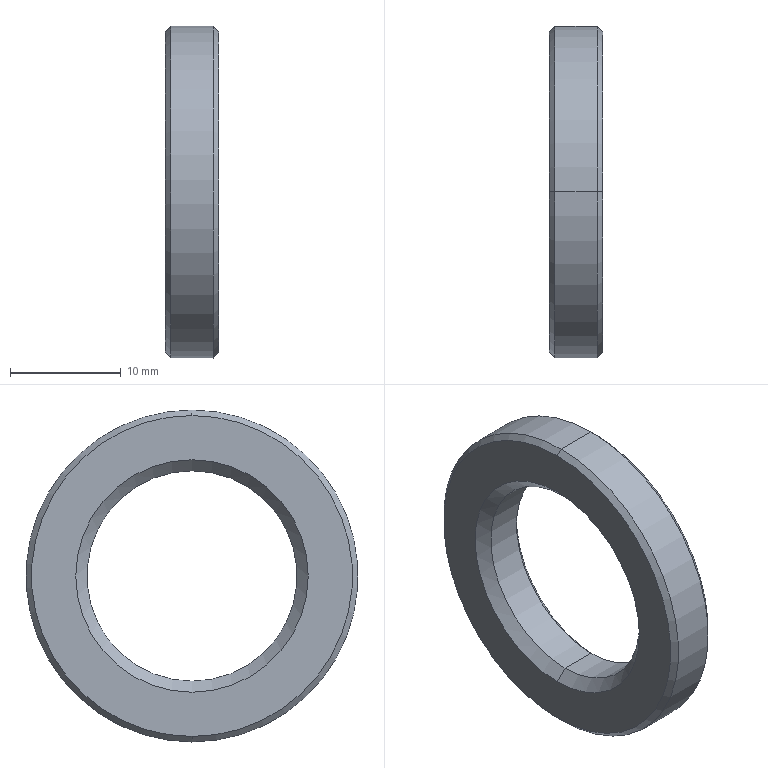Part | SolidWorks | features BaseBody 1 | 1 solid | 26 faces | box 4.8 x 30 x 30 mm | volume 1929 mm3 | cylinder 12 | cone 8 | plane 6 | commonest cylinder face diameters 2.1 x8 19 x2 30 x2
STEP:
#1=CARTESIAN_POINT('',(1.8,0.,15.));
#2=VERTEX_POINT('',#1);
#3=CARTESIAN_POINT('',(1.8,0.,-15.));
#4=VERTEX_POINT('',#3);
#5=CARTESIAN_POINT('',(1.8,0.,0.));
#6=DIRECTION('',(-1.,0.,0.));
#7=DIRECTION('',(0.,0.,1.));
#8=AXIS2_PLACEMENT_3D('',#5,#6,#7);
#9=CIRCLE('',#8,15.);
#10=EDGE_CURVE('',#2,#4,#9,.T.);
#11=ORIENTED_EDGE('',*,*,#10,.T.);
#12=CARTESIAN_POINT('',(-2.,0.,-15.));
#13=VERTEX_POINT('',#12);
#14=CARTESIAN_POINT('',(10.,0.,-15.));
#15=DIRECTION('',(-1.,0.,0.));
#16=VECTOR('',#15,1000.);
#17=LINE('',#14,#16);
#18=EDGE_CURVE('',#4,#13,#17,.T.);
#19=ORIENTED_EDGE('',*,*,#18,.T.);
#20=CARTESIAN_POINT('',(-2.,0.,15.));
#21=VERTEX_POINT('',#20);
#22=CARTESIAN_POINT('',(-2.,0.,0.));
#23=DIRECTION('',(1.,0.,0.));
#24=DIRECTION('',(0.,0.,1.));
#25=AXIS2_PLACEMENT_3D('',#22,#23,#24);
#26=CIRCLE('',#25,15.);
#27=EDGE_CURVE('',#13,#21,#26,.T.);
#28=ORIENTED_EDGE('',*,*,#27,.T.);
#29=CARTESIAN_POINT('',(10.,0.,15.));
#30=DIRECTION('',(-1.,0.,0.));
#31=VECTOR('',#30,1000.);
#32=LINE('',#29,#31);
#33=EDGE_CURVE('',#2,#21,#32,.T.);
#34=ORIENTED_EDGE('',*,*,#33,.F.);
#35=EDGE_LOOP('',(#11,#19,#28,#34));
#36=FACE_OUTER_BOUND('',#35,.T.);
#37=CARTESIAN_POINT('',(10.,0.,0.));
#38=DIRECTION('',(-1.,0.,0.));
#39=DIRECTION('',(0.,0.,1.));
#40=AXIS2_PLACEMENT_3D('',#37,#38,#39);
#41=CYLINDRICAL_SURFACE('',#40,15.);
#42=ADVANCED_FACE('',(#36),#41,.T.);
#43=CARTESIAN_POINT('',(2.3,0.,14.5));
#44=VERTEX_POINT('',#43);
#45=CARTESIAN_POINT('',(2.3,0.,-14.5));
#46=VERTEX_POINT('',#45);
#47=CARTESIAN_POINT('',(2.3,0.,0.));
#48=DIRECTION('',(-1.,0.,0.));
#49=DIRECTION('',(0.,0.,1.));
#50=AXIS2_PLACEMENT_3D('',#47,#48,#49);
#51=CIRCLE('',#50,14.5);
#52=EDGE_CURVE('',#44,#46,#51,.T.);
#53=ORIENTED_EDGE('',*,*,#52,.T.);
#54=CARTESIAN_POINT('',(1.8,0.,-15.));
#55=DIRECTION('',(-0.7071,0.,-0.7071));
#56=VECTOR('',#55,1000.);
#57=LINE('',#54,#56);
#58=EDGE_CURVE('',#46,#4,#57,.T.);
#59=ORIENTED_EDGE('',*,*,#58,.T.);
#60=ORIENTED_EDGE('',*,*,#10,.F.);
#61=CARTESIAN_POINT('',(1.8,0.,15.));
#62=DIRECTION('',(-0.7071,0.,0.7071));
#63=VECTOR('',#62,1000.);
#64=LINE('',#61,#63);
#65=EDGE_CURVE('',#44,#2,#64,.T.);
#66=ORIENTED_EDGE('',*,*,#65,.F.);
#67=EDGE_LOOP('',(#53,#59,#60,#66));
#68=FACE_OUTER_BOUND('',#67,.T.);
#69=CARTESIAN_POINT('',(1.8,0.,0.));
#70=DIRECTION('',(-1.,0.,0.));
#71=DIRECTION('',(0.,0.,1.));
#72=AXIS2_PLACEMENT_3D('',#69,#70,#71);
#73=CONICAL_SURFACE('',#72,15.,0.7854);
#74=ADVANCED_FACE('',(#68),#73,.T.);
#75=CARTESIAN_POINT('',(-2.5,0.,-14.5));
#76=VERTEX_POINT('',#75);
#77=CARTESIAN_POINT('',(-2.5,0.,14.5));
#78=VERTEX_POINT('',#77);
#79=CARTESIAN_POINT('',(-2.5,0.,0.));
#80=DIRECTION('',(1.,0.,0.));
#81=DIRECTION('',(0.,0.,-1.));
#82=AXIS2_PLACEMENT_3D('',#79,#80,#81);
#83=CIRCLE('',#82,14.5);
#84=EDGE_CURVE('',#76,#78,#83,.T.);
#85=ORIENTED_EDGE('',*,*,#84,.T.);
#86=CARTESIAN_POINT('',(-2.,0.,15.));
#87=DIRECTION('',(0.7071,0.,0.7071));
#88=VECTOR('',#87,1000.);
#89=LINE('',#86,#88);
#90=EDGE_CURVE('',#78,#21,#89,.T.);
#91=ORIENTED_EDGE('',*,*,#90,.T.);
#92=ORIENTED_EDGE('',*,*,#27,.F.);
#93=CARTESIAN_POINT('',(-2.,0.,-15.));
#94=DIRECTION('',(0.7071,0.,-0.7071));
#95=VECTOR('',#94,1000.);
#96=LINE('',#93,#95);
#97=EDGE_CURVE('',#76,#13,#96,.T.);
#98=ORIENTED_EDGE('',*,*,#97,.F.);
#99=EDGE_LOOP('',(#85,#91,#92,#98));
#100=FACE_OUTER_BOUND('',#99,.T.);
#101=CARTESIAN_POINT('',(-2.,0.,0.));
#102=DIRECTION('',(1.,0.,0.));
#103=DIRECTION('',(0.,0.,-1.));
#104=AXIS2_PLACEMENT_3D('',#101,#102,#103);
#105=CONICAL_SURFACE('',#104,15.,0.7854);
#106=ADVANCED_FACE('',(#100),#105,.T.);
#107=CARTESIAN_POINT('',(1.8,0.,9.5));
#108=VERTEX_POINT('',#107);
#109=CARTESIAN_POINT('',(1.8,0.,-9.5));
#110=VERTEX_POINT('',#109);
#111=CARTESIAN_POINT('',(1.8,0.,0.));
#112=DIRECTION('',(1.,0.,0.));
#113=DIRECTION('',(0.,0.,-1.));
#114=AXIS2_PLACEMENT_3D('',#111,#112,#113);
#115=CIRCLE('',#114,9.5);
#116=EDGE_CURVE('',#108,#110,#115,.T.);
#117=ORIENTED_EDGE('',*,*,#116,.F.);
#118=CARTESIAN_POINT('',(2.3,0.,10.));
#119=VERTEX_POINT('',#118);
#120=CARTESIAN_POINT('',(2.3,0.,10.));
#121=DIRECTION('',(0.7071,0.,0.7071));
#122=VECTOR('',#121,1000.);
#123=LINE('',#120,#122);
#124=EDGE_CURVE('',#108,#119,#123,.T.);
#125=ORIENTED_EDGE('',*,*,#124,.T.);
#126=CARTESIAN_POINT('',(2.3,0.,-10.));
#127=VERTEX_POINT('',#126);
#128=CARTESIAN_POINT('',(2.3,0.,0.));
#129=DIRECTION('',(-1.,0.,0.));
#130=DIRECTION('',(0.,0.,-1.));
#131=AXIS2_PLACEMENT_3D('',#128,#129,#130);
#132=CIRCLE('',#131,10.);
#133=EDGE_CURVE('',#127,#119,#132,.T.);
#134=ORIENTED_EDGE('',*,*,#133,.F.);
#135=CARTESIAN_POINT('',(2.3,0.,-10.));
#136=DIRECTION('',(0.7071,0.,-0.7071));
#137=VECTOR('',#136,1000.);
#138=LINE('',#135,#137);
#139=EDGE_CURVE('',#110,#127,#138,.T.);
#140=ORIENTED_EDGE('',*,*,#139,.F.);
#141=EDGE_LOOP('',(#117,#125,#134,#140));
#142=FACE_OUTER_BOUND('',#141,.T.);
#143=CARTESIAN_POINT('',(2.3,0.,0.));
#144=DIRECTION('',(1.,0.,0.));
#145=DIRECTION('',(0.,0.,-1.));
#146=AXIS2_PLACEMENT_3D('',#143,#144,#145);
#147=CONICAL_SURFACE('',#146,10.,0.7854);
#148=ADVANCED_FACE('',(#142),#147,.F.);
#149=CARTESIAN_POINT('',(2.3,-12.7,-1.05));
#150=VERTEX_POINT('',#149);
#151=CARTESIAN_POINT('',(2.3,-12.7,1.05));
#152=VERTEX_POINT('',#151);
#153=CARTESIAN_POINT('',(2.3,-12.7,0.));
#154=DIRECTION('',(-1.,0.,0.));
#155=DIRECTION('',(0.,0.,1.));
#156=AXIS2_PLACEMENT_3D('',#153,#154,#155);
#157=CIRCLE('',#156,1.05);
#158=EDGE_CURVE('',#150,#152,#157,.T.);
#159=ORIENTED_EDGE('',*,*,#158,.F.);
#160=CARTESIAN_POINT('',(-0.7,-12.7,-1.05));
#161=VERTEX_POINT('',#160);
#162=CARTESIAN_POINT('',(-0.7,-12.7,-1.05));
#163=DIRECTION('',(-1.,0.,0.));
#164=VECTOR('',#163,1000.);
#165=LINE('',#162,#164);
#166=EDGE_CURVE('',#150,#161,#165,.T.);
#167=ORIENTED_EDGE('',*,*,#166,.T.);
#168=CARTESIAN_POINT('',(-0.7,-12.7,1.05));
#169=VERTEX_POINT('',#168);
#170=CARTESIAN_POINT('',(-0.7,-12.7,0.));
#171=DIRECTION('',(1.,0.,0.));
#172=DIRECTION('',(0.,0.,1.));
#173=AXIS2_PLACEMENT_3D('',#170,#171,#172);
#174=CIRCLE('',#173,1.05);
#175=EDGE_CURVE('',#169,#161,#174,.T.);
#176=ORIENTED_EDGE('',*,*,#175,.F.);
#177=CARTESIAN_POINT('',(-0.7,-12.7,1.05));
#178=DIRECTION('',(-1.,0.,0.));
#179=VECTOR('',#178,1000.);
#180=LINE('',#177,#179);
#181=EDGE_CURVE('',#152,#169,#180,.T.);
#182=ORIENTED_EDGE('',*,*,#181,.F.);
#183=EDGE_LOOP('',(#159,#167,#176,#182));
#184=FACE_OUTER_BOUND('',#183,.T.);
#185=CARTESIAN_POINT('',(-0.7,-12.7,0.));
#186=DIRECTION('',(-1.,0.,0.));
#187=DIRECTION('',(0.,0.,1.));
#188=AXIS2_PLACEMENT_3D('',#185,#186,#187);
#189=CYLINDRICAL_SURFACE('',#188,1.05);
#190=ADVANCED_FACE('',(#184),#189,.F.);
#191=CARTESIAN_POINT('',(2.3,0.,-13.75));
#192=VERTEX_POINT('',#191);
#193=CARTESIAN_POINT('',(2.3,0.,-11.65));
#194=VERTEX_POINT('',#193);
#195=CARTESIAN_POINT('',(2.3,0.,-12.7));
#196=DIRECTION('',(-1.,0.,0.));
#197=DIRECTION('',(0.,0.,1.));
#198=AXIS2_PLACEMENT_3D('',#195,#196,#197);
#199=CIRCLE('',#198,1.05);
#200=EDGE_CURVE('',#192,#194,#199,.T.);
#201=ORIENTED_EDGE('',*,*,#200,.F.);
#202=CARTESIAN_POINT('',(-0.7,0.,-13.75));
#203=VERTEX_POINT('',#202);
#204=CARTESIAN_POINT('',(-0.7,0.,-13.75));
#205=DIRECTION('',(-1.,0.,0.));
#206=VECTOR('',#205,1000.);
#207=LINE('',#204,#206);
#208=EDGE_CURVE('',#192,#203,#207,.T.);
#209=ORIENTED_EDGE('',*,*,#208,.T.);
#210=CARTESIAN_POINT('',(-0.7,0.,-11.65));
#211=VERTEX_POINT('',#210);
#212=CARTESIAN_POINT('',(-0.7,0.,-12.7));
#213=DIRECTION('',(1.,0.,0.));
#214=DIRECTION('',(0.,0.,1.));
#215=AXIS2_PLACEMENT_3D('',#212,#213,#214);
#216=CIRCLE('',#215,1.05);
#217=EDGE_CURVE('',#211,#203,#216,.T.);
#218=ORIENTED_EDGE('',*,*,#217,.F.);
#219=CARTESIAN_POINT('',(-0.7,0.,-11.65));
#220=DIRECTION('',(-1.,0.,0.));
#221=VECTOR('',#220,1000.);
#222=LINE('',#219,#221);
#223=EDGE_CURVE('',#194,#211,#222,.T.);
#224=ORIENTED_EDGE('',*,*,#223,.F.);
#225=EDGE_LOOP('',(#201,#209,#218,#224));
#226=FACE_OUTER_BOUND('',#225,.T.);
#227=CARTESIAN_POINT('',(-0.7,0.,-12.7));
#228=DIRECTION('',(-1.,0.,0.));
#229=DIRECTION('',(0.,0.,1.));
#230=AXIS2_PLACEMENT_3D('',#227,#228,#229);
#231=CYLINDRICAL_SURFACE('',#230,1.05);
#232=ADVANCED_FACE('',(#226),#231,.F.);
#233=CARTESIAN_POINT('',(2.3,0.,11.65));
#234=VERTEX_POINT('',#233);
#235=CARTESIAN_POINT('',(2.3,0.,13.75));
#236=VERTEX_POINT('',#235);
#237=CARTESIAN_POINT('',(2.3,0.,12.7));
#238=DIRECTION('',(-1.,0.,0.));
#239=DIRECTION('',(0.,0.,1.));
#240=AXIS2_PLACEMENT_3D('',#237,#238,#239);
#241=CIRCLE('',#240,1.05);
#242=EDGE_CURVE('',#234,#236,#241,.T.);
#243=ORIENTED_EDGE('',*,*,#242,.F.);
#244=CARTESIAN_POINT('',(-0.7,0.,11.65));
#245=VERTEX_POINT('',#244);
#246=CARTESIAN_POINT('',(-0.7,0.,11.65));
#247=DIRECTION('',(-1.,0.,0.));
#248=VECTOR('',#247,1000.);
#249=LINE('',#246,#248);
#250=EDGE_CURVE('',#234,#245,#249,.T.);
#251=ORIENTED_EDGE('',*,*,#250,.T.);
#252=CARTESIAN_POINT('',(-0.7,0.,13.75));
#253=VERTEX_POINT('',#252);
#254=CARTESIAN_POINT('',(-0.7,0.,12.7));
#255=DIRECTION('',(1.,0.,0.));
#256=DIRECTION('',(0.,0.,1.));
#257=AXIS2_PLACEMENT_3D('',#254,#255,#256);
#258=CIRCLE('',#257,1.05);
#259=EDGE_CURVE('',#253,#245,#258,.T.);
#260=ORIENTED_EDGE('',*,*,#259,.F.);
#261=CARTESIAN_POINT('',(-0.7,0.,13.75));
#262=DIRECTION('',(-1.,0.,0.));
#263=VECTOR('',#262,1000.);
#264=LINE('',#261,#263);
#265=EDGE_CURVE('',#236,#253,#264,.T.);
#266=ORIENTED_EDGE('',*,*,#265,.F.);
#267=EDGE_LOOP('',(#243,#251,#260,#266));
#268=FACE_OUTER_BOUND('',#267,.T.);
#269=CARTESIAN_POINT('',(-0.7,0.,12.7));
#270=DIRECTION('',(-1.,0.,0.));
#271=DIRECTION('',(0.,0.,1.));
#272=AXIS2_PLACEMENT_3D('',#269,#270,#271);
#273=CYLINDRICAL_SURFACE('',#272,1.05);
#274=ADVANCED_FACE('',(#268),#273,.F.);
#275=CARTESIAN_POINT('',(2.3,12.7,-1.05));
#276=VERTEX_POINT('',#275);
#277=CARTESIAN_POINT('',(2.3,12.7,1.05));
#278=VERTEX_POINT('',#277);
#279=CARTESIAN_POINT('',(2.3,12.7,0.));
#280=DIRECTION('',(-1.,0.,0.));
#281=DIRECTION('',(0.,0.,1.));
#282=AXIS2_PLACEMENT_3D('',#279,#280,#281);
#283=CIRCLE('',#282,1.05);
#284=EDGE_CURVE('',#276,#278,#283,.T.);
#285=ORIENTED_EDGE('',*,*,#284,.F.);
#286=CARTESIAN_POINT('',(-0.7,12.7,-1.05));
#287=VERTEX_POINT('',#286);
#288=CARTESIAN_POINT('',(-0.7,12.7,-1.05));
#289=DIRECTION('',(-1.,0.,0.));
#290=VECTOR('',#289,1000.);
#291=LINE('',#288,#290);
#292=EDGE_CURVE('',#276,#287,#291,.T.);
#293=ORIENTED_EDGE('',*,*,#292,.T.);
#294=CARTESIAN_POINT('',(-0.7,12.7,1.05));
#295=VERTEX_POINT('',#294);
#296=CARTESIAN_POINT('',(-0.7,12.7,0.));
#297=DIRECTION('',(1.,0.,0.));
#298=DIRECTION('',(0.,0.,1.));
#299=AXIS2_PLACEMENT_3D('',#296,#297,#298);
#300=CIRCLE('',#299,1.05);
#301=EDGE_CURVE('',#295,#287,#300,.T.);
#302=ORIENTED_EDGE('',*,*,#301,.F.);
#303=CARTESIAN_POINT('',(-0.7,12.7,1.05));
#304=DIRECTION('',(-1.,0.,0.));
#305=VECTOR('',#304,1000.);
#306=LINE('',#303,#305);
#307=EDGE_CURVE('',#278,#295,#306,.T.);
#308=ORIENTED_EDGE('',*,*,#307,.F.);
#309=EDGE_LOOP('',(#285,#293,#302,#308));
#310=FACE_OUTER_BOUND('',#309,.T.);
#311=CARTESIAN_POINT('',(-0.7,12.7,0.));
#312=DIRECTION('',(-1.,0.,0.));
#313=DIRECTION('',(0.,0.,1.));
#314=AXIS2_PLACEMENT_3D('',#311,#312,#313);
#315=CYLINDRICAL_SURFACE('',#314,1.05);
#316=ADVANCED_FACE('',(#310),#315,.F.);
#317=CARTESIAN_POINT('',(-1.5,0.,-9.5));
#318=VERTEX_POINT('',#317);
#319=CARTESIAN_POINT('',(-1.5,0.,9.5));
#320=VERTEX_POINT('',#319);
#321=CARTESIAN_POINT('',(-1.5,0.,0.));
#322=DIRECTION('',(-1.,0.,0.));
#323=DIRECTION('',(0.,0.,1.));
#324=AXIS2_PLACEMENT_3D('',#321,#322,#323);
#325=CIRCLE('',#324,9.5);
#326=EDGE_CURVE('',#318,#320,#325,.T.);
#327=ORIENTED_EDGE('',*,*,#326,.F.);
#328=CARTESIAN_POINT('',(-2.5,0.,-10.5));
#329=VERTEX_POINT('',#328);
#330=CARTESIAN_POINT('',(-2.5,0.,-10.5));
#331=DIRECTION('',(-0.7071,0.,-0.7071));
#332=VECTOR('',#331,1000.);
#333=LINE('',#330,#332);
#334=EDGE_CURVE('',#318,#329,#333,.T.);
#335=ORIENTED_EDGE('',*,*,#334,.T.);
#336=CARTESIAN_POINT('',(-2.5,0.,10.5));
#337=VERTEX_POINT('',#336);
#338=CARTESIAN_POINT('',(-2.5,0.,0.));
#339=DIRECTION('',(1.,0.,0.));
#340=DIRECTION('',(0.,0.,1.));
#341=AXIS2_PLACEMENT_3D('',#338,#339,#340);
#342=CIRCLE('',#341,10.5);
#343=EDGE_CURVE('',#337,#329,#342,.T.);
#344=ORIENTED_EDGE('',*,*,#343,.F.);
#345=CARTESIAN_POINT('',(-2.5,0.,10.5));
#346=DIRECTION('',(-0.7071,0.,0.7071));
#347=VECTOR('',#346,1000.);
#348=LINE('',#345,#347);
#349=EDGE_CURVE('',#320,#337,#348,.T.);
#350=ORIENTED_EDGE('',*,*,#349,.F.);
#351=EDGE_LOOP('',(#327,#335,#344,#350));
#352=FACE_OUTER_BOUND('',#351,.T.);
#353=CARTESIAN_POINT('',(-2.5,0.,0.));
#354=DIRECTION('',(-1.,0.,0.));
#355=DIRECTION('',(0.,0.,1.));
#356=AXIS2_PLACEMENT_3D('',#353,#354,#355);
#357=CONICAL_SURFACE('',#356,10.5,0.7854);
#358=ADVANCED_FACE('',(#352),#357,.F.);
#359=ORIENTED_EDGE('',*,*,#116,.T.);
#360=CARTESIAN_POINT('',(10.,0.,-9.5));
#361=DIRECTION('',(-1.,0.,0.));
#362=VECTOR('',#361,1000.);
#363=LINE('',#360,#362);
#364=EDGE_CURVE('',#110,#318,#363,.T.);
#365=ORIENTED_EDGE('',*,*,#364,.T.);
#366=ORIENTED_EDGE('',*,*,#326,.T.);
#367=CARTESIAN_POINT('',(10.,0.,9.5));
#368=DIRECTION('',(-1.,0.,0.));
#369=VECTOR('',#368,1000.);
#370=LINE('',#367,#369);
#371=EDGE_CURVE('',#108,#320,#370,.T.);
#372=ORIENTED_EDGE('',*,*,#371,.F.);
#373=EDGE_LOOP('',(#359,#365,#366,#372));
#374=FACE_OUTER_BOUND('',#373,.T.);
#375=CARTESIAN_POINT('',(10.,0.,0.));
#376=DIRECTION('',(-1.,0.,0.));
#377=DIRECTION('',(0.,0.,1.));
#378=AXIS2_PLACEMENT_3D('',#375,#376,#377);
#379=CYLINDRICAL_SURFACE('',#378,9.5);
#380=ADVANCED_FACE('',(#374),#379,.F.);
#381=ORIENTED_EDGE('',*,*,#18,.F.);
#382=CARTESIAN_POINT('',(1.8,0.,0.));
#383=DIRECTION('',(-1.,0.,0.));
#384=DIRECTION('',(0.,0.,1.));
#385=AXIS2_PLACEMENT_3D('',#382,#383,#384);
#386=CIRCLE('',#385,15.);
#387=EDGE_CURVE('',#4,#2,#386,.T.);
#388=ORIENTED_EDGE('',*,*,#387,.T.);
#389=ORIENTED_EDGE('',*,*,#33,.T.);
#390=CARTESIAN_POINT('',(-2.,0.,0.));
#391=DIRECTION('',(1.,0.,0.));
#392=DIRECTION('',(0.,0.,1.));
#393=AXIS2_PLACEMENT_3D('',#390,#391,#392);
#394=CIRCLE('',#393,15.);
#395=EDGE_CURVE('',#21,#13,#394,.T.);
#396=ORIENTED_EDGE('',*,*,#395,.T.);
#397=EDGE_LOOP('',(#381,#388,#389,#396));
#398=FACE_OUTER_BOUND('',#397,.T.);
#399=CARTESIAN_POINT('',(10.,0.,0.));
#400=DIRECTION('',(-1.,0.,0.));
#401=DIRECTION('',(0.,0.,1.));
#402=AXIS2_PLACEMENT_3D('',#399,#400,#401);
#403=CYLINDRICAL_SURFACE('',#402,15.);
#404=ADVANCED_FACE('',(#398),#403,.T.);
#405=ORIENTED_EDGE('',*,*,#58,.F.);
#406=CARTESIAN_POINT('',(2.3,0.,0.));
#407=DIRECTION('',(-1.,0.,0.));
#408=DIRECTION('',(0.,0.,1.));
#409=AXIS2_PLACEMENT_3D('',#406,#407,#408);
#410=CIRCLE('',#409,14.5);
#411=EDGE_CURVE('',#46,#44,#410,.T.);
#412=ORIENTED_EDGE('',*,*,#411,.T.);
#413=ORIENTED_EDGE('',*,*,#65,.T.);
#414=ORIENTED_EDGE('',*,*,#387,.F.);
#415=EDGE_LOOP('',(#405,#412,#413,#414));
#416=FACE_OUTER_BOUND('',#415,.T.);
#417=CARTESIAN_POINT('',(1.8,0.,0.));
#418=DIRECTION('',(-1.,0.,0.));
#419=DIRECTION('',(0.,0.,1.));
#420=AXIS2_PLACEMENT_3D('',#417,#418,#419);
#421=CONICAL_SURFACE('',#420,15.,0.7854);
#422=ADVANCED_FACE('',(#416),#421,.T.);
#423=ORIENTED_EDGE('',*,*,#90,.F.);
#424=CARTESIAN_POINT('',(-2.5,0.,0.));
#425=DIRECTION('',(1.,0.,0.));
#426=DIRECTION('',(0.,0.,-1.));
#427=AXIS2_PLACEMENT_3D('',#424,#425,#426);
#428=CIRCLE('',#427,14.5);
#429=EDGE_CURVE('',#78,#76,#428,.T.);
#430=ORIENTED_EDGE('',*,*,#429,.T.);
#431=ORIENTED_EDGE('',*,*,#97,.T.);
#432=ORIENTED_EDGE('',*,*,#395,.F.);
#433=EDGE_LOOP('',(#423,#430,#431,#432));
#434=FACE_OUTER_BOUND('',#433,.T.);
#435=CARTESIAN_POINT('',(-2.,0.,0.));
#436=DIRECTION('',(1.,0.,0.));
#437=DIRECTION('',(0.,0.,-1.));
#438=AXIS2_PLACEMENT_3D('',#435,#436,#437);
#439=CONICAL_SURFACE('',#438,15.,0.7854);
#440=ADVANCED_FACE('',(#434),#439,.T.);
#441=ORIENTED_EDGE('',*,*,#133,.T.);
#442=CARTESIAN_POINT('',(2.3,0.,0.));
#443=DIRECTION('',(-1.,0.,0.));
#444=DIRECTION('',(0.,0.,-1.));
#445=AXIS2_PLACEMENT_3D('',#442,#443,#444);
#446=CIRCLE('',#445,10.);
#447=EDGE_CURVE('',#119,#127,#446,.T.);
#448=ORIENTED_EDGE('',*,*,#447,.T.);
#449=EDGE_LOOP('',(#441,#448));
#450=FACE_BOUND('',#449,.T.);
#451=CARTESIAN_POINT('',(2.3,-12.7,0.));
#452=DIRECTION('',(-1.,0.,0.));
#453=DIRECTION('',(0.,0.,1.));
#454=AXIS2_PLACEMENT_3D('',#451,#452,#453);
#455=CIRCLE('',#454,1.05);
#456=EDGE_CURVE('',#152,#150,#455,.T.);
#457=ORIENTED_EDGE('',*,*,#456,.T.);
#458=ORIENTED_EDGE('',*,*,#158,.T.);
#459=EDGE_LOOP('',(#457,#458));
#460=FACE_BOUND('',#459,.T.);
#461=CARTESIAN_POINT('',(2.3,0.,-12.7));
#462=DIRECTION('',(-1.,0.,0.));
#463=DIRECTION('',(0.,0.,1.));
#464=AXIS2_PLACEMENT_3D('',#461,#462,#463);
#465=CIRCLE('',#464,1.05);
#466=EDGE_CURVE('',#194,#192,#465,.T.);
#467=ORIENTED_EDGE('',*,*,#466,.T.);
#468=ORIENTED_EDGE('',*,*,#200,.T.);
#469=EDGE_LOOP('',(#467,#468));
#470=FACE_BOUND('',#469,.T.);
#471=CARTESIAN_POINT('',(2.3,0.,12.7));
#472=DIRECTION('',(-1.,0.,0.));
#473=DIRECTION('',(0.,0.,1.));
#474=AXIS2_PLACEMENT_3D('',#471,#472,#473);
#475=CIRCLE('',#474,1.05);
#476=EDGE_CURVE('',#236,#234,#475,.T.);
#477=ORIENTED_EDGE('',*,*,#476,.T.);
#478=ORIENTED_EDGE('',*,*,#242,.T.);
#479=EDGE_LOOP('',(#477,#478));
#480=FACE_BOUND('',#479,.T.);
#481=CARTESIAN_POINT('',(2.3,12.7,0.));
#482=DIRECTION('',(-1.,0.,0.));
#483=DIRECTION('',(0.,0.,1.));
#484=AXIS2_PLACEMENT_3D('',#481,#482,#483);
#485=CIRCLE('',#484,1.05);
#486=EDGE_CURVE('',#278,#276,#485,.T.);
#487=ORIENTED_EDGE('',*,*,#486,.T.);
#488=ORIENTED_EDGE('',*,*,#284,.T.);
#489=EDGE_LOOP('',(#487,#488));
#490=FACE_BOUND('',#489,.T.);
#491=ORIENTED_EDGE('',*,*,#52,.F.);
#492=ORIENTED_EDGE('',*,*,#411,.F.);
#493=EDGE_LOOP('',(#491,#492));
#494=FACE_OUTER_BOUND('',#493,.T.);
#495=CARTESIAN_POINT('',(2.3,10.,0.));
#496=DIRECTION('',(1.,0.,0.));
#497=DIRECTION('',(0.,0.,-1.));
#498=AXIS2_PLACEMENT_3D('',#495,#496,#497);
#499=PLANE('',#498);
#500=ADVANCED_FACE('',(#450,#460,#470,#480,#490,#494),#499,.T.);
#501=ORIENTED_EDGE('',*,*,#84,.F.);
#502=ORIENTED_EDGE('',*,*,#429,.F.);
#503=EDGE_LOOP('',(#501,#502));
#504=FACE_OUTER_BOUND('',#503,.T.);
#505=ORIENTED_EDGE('',*,*,#343,.T.);
#506=CARTESIAN_POINT('',(-2.5,0.,0.));
#507=DIRECTION('',(1.,0.,0.));
#508=DIRECTION('',(0.,0.,1.));
#509=AXIS2_PLACEMENT_3D('',#506,#507,#508);
#510=CIRCLE('',#509,10.5);
#511=EDGE_CURVE('',#329,#337,#510,.T.);
#512=ORIENTED_EDGE('',*,*,#511,.T.);
#513=EDGE_LOOP('',(#505,#512));
#514=FACE_BOUND('',#513,.T.);
#515=CARTESIAN_POINT('',(-2.5,14.5,0.));
#516=DIRECTION('',(-1.,0.,0.));
#517=DIRECTION('',(0.,0.,1.));
#518=AXIS2_PLACEMENT_3D('',#515,#516,#517);
#519=PLANE('',#518);
#520=ADVANCED_FACE('',(#504,#514),#519,.T.);
#521=ORIENTED_EDGE('',*,*,#124,.F.);
#522=CARTESIAN_POINT('',(1.8,0.,0.));
#523=DIRECTION('',(1.,0.,0.));
#524=DIRECTION('',(0.,0.,-1.));
#525=AXIS2_PLACEMENT_3D('',#522,#523,#524);
#526=CIRCLE('',#525,9.5);
#527=EDGE_CURVE('',#110,#108,#526,.T.);
#528=ORIENTED_EDGE('',*,*,#527,.F.);
#529=ORIENTED_EDGE('',*,*,#139,.T.);
#530=ORIENTED_EDGE('',*,*,#447,.F.);
#531=EDGE_LOOP('',(#521,#528,#529,#530));
#532=FACE_OUTER_BOUND('',#531,.T.);
#533=CARTESIAN_POINT('',(2.3,0.,0.));
#534=DIRECTION('',(1.,0.,0.));
#535=DIRECTION('',(0.,0.,-1.));
#536=AXIS2_PLACEMENT_3D('',#533,#534,#535);
#537=CONICAL_SURFACE('',#536,10.,0.7854);
#538=ADVANCED_FACE('',(#532),#537,.F.);
#539=ORIENTED_EDGE('',*,*,#166,.F.);
#540=ORIENTED_EDGE('',*,*,#456,.F.);
#541=ORIENTED_EDGE('',*,*,#181,.T.);
#542=CARTESIAN_POINT('',(-0.7,-12.7,0.));
#543=DIRECTION('',(1.,0.,0.));
#544=DIRECTION('',(0.,0.,1.));
#545=AXIS2_PLACEMENT_3D('',#542,#543,#544);
#546=CIRCLE('',#545,1.05);
#547=EDGE_CURVE('',#161,#169,#546,.T.);
#548=ORIENTED_EDGE('',*,*,#547,.F.);
#549=EDGE_LOOP('',(#539,#540,#541,#548));
#550=FACE_OUTER_BOUND('',#549,.T.);
#551=CARTESIAN_POINT('',(-0.7,-12.7,0.));
#552=DIRECTION('',(-1.,0.,0.));
#553=DIRECTION('',(0.,0.,1.));
#554=AXIS2_PLACEMENT_3D('',#551,#552,#553);
#555=CYLINDRICAL_SURFACE('',#554,1.05);
#556=ADVANCED_FACE('',(#550),#555,.F.);
#557=ORIENTED_EDGE('',*,*,#208,.F.);
#558=ORIENTED_EDGE('',*,*,#466,.F.);
#559=ORIENTED_EDGE('',*,*,#223,.T.);
#560=CARTESIAN_POINT('',(-0.7,0.,-12.7));
#561=DIRECTION('',(1.,0.,0.));
#562=DIRECTION('',(0.,0.,1.));
#563=AXIS2_PLACEMENT_3D('',#560,#561,#562);
#564=CIRCLE('',#563,1.05);
#565=EDGE_CURVE('',#203,#211,#564,.T.);
#566=ORIENTED_EDGE('',*,*,#565,.F.);
#567=EDGE_LOOP('',(#557,#558,#559,#566));
#568=FACE_OUTER_BOUND('',#567,.T.);
#569=CARTESIAN_POINT('',(-0.7,0.,-12.7));
#570=DIRECTION('',(-1.,0.,0.));
#571=DIRECTION('',(0.,0.,1.));
#572=AXIS2_PLACEMENT_3D('',#569,#570,#571);
#573=CYLINDRICAL_SURFACE('',#572,1.05);
#574=ADVANCED_FACE('',(#568),#573,.F.);
#575=ORIENTED_EDGE('',*,*,#250,.F.);
#576=ORIENTED_EDGE('',*,*,#476,.F.);
#577=ORIENTED_EDGE('',*,*,#265,.T.);
#578=CARTESIAN_POINT('',(-0.7,0.,12.7));
#579=DIRECTION('',(1.,0.,0.));
#580=DIRECTION('',(0.,0.,1.));
#581=AXIS2_PLACEMENT_3D('',#578,#579,#580);
#582=CIRCLE('',#581,1.05);
#583=EDGE_CURVE('',#245,#253,#582,.T.);
#584=ORIENTED_EDGE('',*,*,#583,.F.);
#585=EDGE_LOOP('',(#575,#576,#577,#584));
#586=FACE_OUTER_BOUND('',#585,.T.);
#587=CARTESIAN_POINT('',(-0.7,0.,12.7));
#588=DIRECTION('',(-1.,0.,0.));
#589=DIRECTION('',(0.,0.,1.));
#590=AXIS2_PLACEMENT_3D('',#587,#588,#589);
#591=CYLINDRICAL_SURFACE('',#590,1.05);
#592=ADVANCED_FACE('',(#586),#591,.F.);
#593=ORIENTED_EDGE('',*,*,#292,.F.);
#594=ORIENTED_EDGE('',*,*,#486,.F.);
#595=ORIENTED_EDGE('',*,*,#307,.T.);
#596=CARTESIAN_POINT('',(-0.7,12.7,0.));
#597=DIRECTION('',(1.,0.,0.));
#598=DIRECTION('',(0.,0.,1.));
#599=AXIS2_PLACEMENT_3D('',#596,#597,#598);
#600=CIRCLE('',#599,1.05);
#601=EDGE_CURVE('',#287,#295,#600,.T.);
#602=ORIENTED_EDGE('',*,*,#601,.F.);
#603=EDGE_LOOP('',(#593,#594,#595,#602));
#604=FACE_OUTER_BOUND('',#603,.T.);
#605=CARTESIAN_POINT('',(-0.7,12.7,0.));
#606=DIRECTION('',(-1.,0.,0.));
#607=DIRECTION('',(0.,0.,1.));
#608=AXIS2_PLACEMENT_3D('',#605,#606,#607);
#609=CYLINDRICAL_SURFACE('',#608,1.05);
#610=ADVANCED_FACE('',(#604),#609,.F.);
#611=ORIENTED_EDGE('',*,*,#334,.F.);
#612=CARTESIAN_POINT('',(-1.5,0.,0.));
#613=DIRECTION('',(-1.,0.,0.));
#614=DIRECTION('',(0.,0.,1.));
#615=AXIS2_PLACEMENT_3D('',#612,#613,#614);
#616=CIRCLE('',#615,9.5);
#617=EDGE_CURVE('',#320,#318,#616,.T.);
#618=ORIENTED_EDGE('',*,*,#617,.F.);
#619=ORIENTED_EDGE('',*,*,#349,.T.);
#620=ORIENTED_EDGE('',*,*,#511,.F.);
#621=EDGE_LOOP('',(#611,#618,#619,#620));
#622=FACE_OUTER_BOUND('',#621,.T.);
#623=CARTESIAN_POINT('',(-2.5,0.,0.));
#624=DIRECTION('',(-1.,0.,0.));
#625=DIRECTION('',(0.,0.,1.));
#626=AXIS2_PLACEMENT_3D('',#623,#624,#625);
#627=CONICAL_SURFACE('',#626,10.5,0.7854);
#628=ADVANCED_FACE('',(#622),#627,.F.);
#629=ORIENTED_EDGE('',*,*,#364,.F.);
#630=ORIENTED_EDGE('',*,*,#527,.T.);
#631=ORIENTED_EDGE('',*,*,#371,.T.);
#632=ORIENTED_EDGE('',*,*,#617,.T.);
#633=EDGE_LOOP('',(#629,#630,#631,#632));
#634=FACE_OUTER_BOUND('',#633,.T.);
#635=CARTESIAN_POINT('',(10.,0.,0.));
#636=DIRECTION('',(-1.,0.,0.));
#637=DIRECTION('',(0.,0.,1.));
#638=AXIS2_PLACEMENT_3D('',#635,#636,#637);
#639=CYLINDRICAL_SURFACE('',#638,9.5);
#640=ADVANCED_FACE('',(#634),#639,.F.);
#641=ORIENTED_EDGE('',*,*,#175,.T.);
#642=ORIENTED_EDGE('',*,*,#547,.T.);
#643=EDGE_LOOP('',(#641,#642));
#644=FACE_OUTER_BOUND('',#643,.T.);
#645=CARTESIAN_POINT('',(-0.7,-12.7,0.));
#646=DIRECTION('',(1.,0.,0.));
#647=DIRECTION('',(0.,0.,-1.));
#648=AXIS2_PLACEMENT_3D('',#645,#646,#647);
#649=PLANE('',#648);
#650=ADVANCED_FACE('',(#644),#649,.T.);
#651=ORIENTED_EDGE('',*,*,#217,.T.);
#652=ORIENTED_EDGE('',*,*,#565,.T.);
#653=EDGE_LOOP('',(#651,#652));
#654=FACE_OUTER_BOUND('',#653,.T.);
#655=CARTESIAN_POINT('',(-0.7,0.,-12.7));
#656=DIRECTION('',(1.,0.,0.));
#657=DIRECTION('',(0.,0.,-1.));
#658=AXIS2_PLACEMENT_3D('',#655,#656,#657);
#659=PLANE('',#658);
#660=ADVANCED_FACE('',(#654),#659,.T.);
#661=ORIENTED_EDGE('',*,*,#259,.T.);
#662=ORIENTED_EDGE('',*,*,#583,.T.);
#663=EDGE_LOOP('',(#661,#662));
#664=FACE_OUTER_BOUND('',#663,.T.);
#665=CARTESIAN_POINT('',(-0.7,0.,12.7));
#666=DIRECTION('',(1.,0.,0.));
#667=DIRECTION('',(0.,0.,-1.));
#668=AXIS2_PLACEMENT_3D('',#665,#666,#667);
#669=PLANE('',#668);
#670=ADVANCED_FACE('',(#664),#669,.T.);
#671=ORIENTED_EDGE('',*,*,#301,.T.);
#672=ORIENTED_EDGE('',*,*,#601,.T.);
#673=EDGE_LOOP('',(#671,#672));
#674=FACE_OUTER_BOUND('',#673,.T.);
#675=CARTESIAN_POINT('',(-0.7,12.7,0.));
#676=DIRECTION('',(1.,0.,0.));
#677=DIRECTION('',(0.,0.,-1.));
#678=AXIS2_PLACEMENT_3D('',#675,#676,#677);
#679=PLANE('',#678);
#680=ADVANCED_FACE('',(#674),#679,.T.);
#681=CLOSED_SHELL('',(#42,#74,#106,#148,#190,#232,#274,#316,#358,#380,#404,#422,#440,#500,#520,#538,#556,#574,#592,#610,#628,#640,#650,#660,#670,#680));
#682=MANIFOLD_SOLID_BREP('',#681);
#683=CARTESIAN_POINT('',(0.,0.,0.));
#684=DIRECTION('',(0.,0.,1.));
#685=DIRECTION('',(1.,0.,0.));
#686=AXIS2_PLACEMENT_3D('',#683,#684,#685);
#687=(LENGTH_UNIT()NAMED_UNIT(*)SI_UNIT(.MILLI.,.METRE.));
#688=UNCERTAINTY_MEASURE_WITH_UNIT(LENGTH_MEASURE(0.00001),#687,'','');
#689=(NAMED_UNIT(*)PLANE_ANGLE_UNIT()SI_UNIT($,.RADIAN.));
#690=(NAMED_UNIT(*)SI_UNIT($,.STERADIAN.)SOLID_ANGLE_UNIT());
#691=(GEOMETRIC_REPRESENTATION_CONTEXT(3)GLOBAL_UNCERTAINTY_ASSIGNED_CONTEXT((#688))GLOBAL_UNIT_ASSIGNED_CONTEXT((#687,#689,#690))REPRESENTATION_CONTEXT('',''));
#692=ADVANCED_BREP_SHAPE_REPRESENTATION('',(#682,#686),#691);